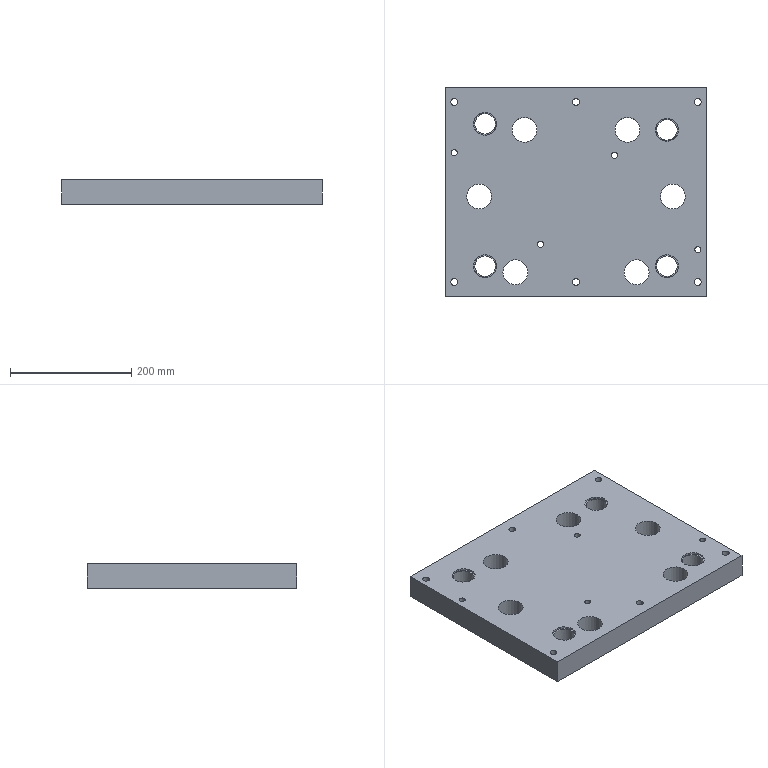Part | NX | features solid 2 | 1 solid | 94 faces | box 430 x 345.001 x 40 mm | volume 5387052 mm3 | cylinder 48 | plane 24 | cone 22 | commonest cylinder face diameters 8.5 x6 11.507 x6 12 x6 18.008 x6 41 x6 8.506 x4